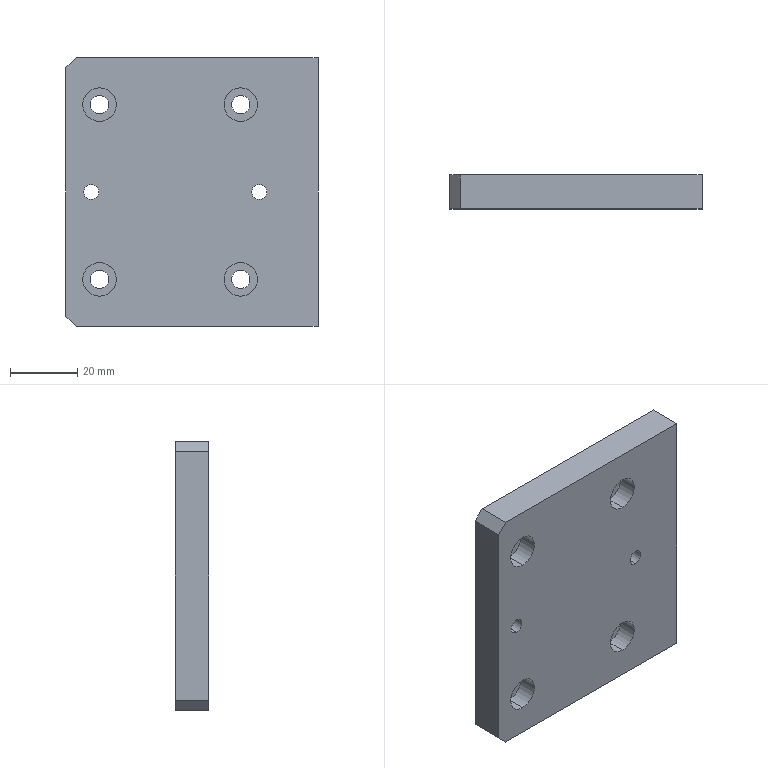Part | SolidWorks | features HoleWzd 3, Chamfer 1, Extrusion 1 | 1 solid | 46 faces | box 75 x 10 x 80 mm | volume 56721 mm3 | cylinder 28 | plane 14 | cone 4 | commonest cylinder face diameters 5.5 x8 10 x8 4.2 x4 4.5 x4 8 x4
STEP:
#1=CARTESIAN_POINT('',(-30.,0.4,-4.));
#2=VERTEX_POINT('',#1);
#3=CARTESIAN_POINT('',(-30.,0.4,4.));
#4=VERTEX_POINT('',#3);
#5=CARTESIAN_POINT('',(-30.,0.4,0.));
#6=DIRECTION('',(0.,1.,0.));
#7=DIRECTION('',(0.,0.,1.));
#8=AXIS2_PLACEMENT_3D('',#5,#6,#7);
#9=CIRCLE('',#8,4.);
#10=EDGE_CURVE('',#2,#4,#9,.T.);
#11=ORIENTED_EDGE('',*,*,#10,.F.);
#12=CARTESIAN_POINT('',(-30.,5.,-4.));
#13=VERTEX_POINT('',#12);
#14=CARTESIAN_POINT('',(-30.,5.,-4.));
#15=DIRECTION('',(0.,1.,0.));
#16=VECTOR('',#15,1000.);
#17=LINE('',#14,#16);
#18=EDGE_CURVE('',#2,#13,#17,.T.);
#19=ORIENTED_EDGE('',*,*,#18,.T.);
#20=CARTESIAN_POINT('',(-30.,5.,4.));
#21=VERTEX_POINT('',#20);
#22=CARTESIAN_POINT('',(-30.,5.,0.));
#23=DIRECTION('',(0.,1.,0.));
#24=DIRECTION('',(0.,0.,1.));
#25=AXIS2_PLACEMENT_3D('',#22,#23,#24);
#26=CIRCLE('',#25,4.);
#27=EDGE_CURVE('',#13,#21,#26,.T.);
#28=ORIENTED_EDGE('',*,*,#27,.T.);
#29=CARTESIAN_POINT('',(-30.,5.,4.));
#30=DIRECTION('',(0.,1.,0.));
#31=VECTOR('',#30,1000.);
#32=LINE('',#29,#31);
#33=EDGE_CURVE('',#4,#21,#32,.T.);
#34=ORIENTED_EDGE('',*,*,#33,.F.);
#35=EDGE_LOOP('',(#11,#19,#28,#34));
#36=FACE_OUTER_BOUND('',#35,.T.);
#37=CARTESIAN_POINT('',(-30.,5.,0.));
#38=DIRECTION('',(0.,1.,0.));
#39=DIRECTION('',(0.,0.,1.));
#40=AXIS2_PLACEMENT_3D('',#37,#38,#39);
#41=CYLINDRICAL_SURFACE('',#40,4.);
#42=ADVANCED_FACE('',(#36),#41,.F.);
#43=CARTESIAN_POINT('',(-30.,-5.,-2.25));
#44=VERTEX_POINT('',#43);
#45=CARTESIAN_POINT('',(-30.,-5.,2.25));
#46=VERTEX_POINT('',#45);
#47=CARTESIAN_POINT('',(-30.,-5.,0.));
#48=DIRECTION('',(0.,1.,0.));
#49=DIRECTION('',(0.,0.,1.));
#50=AXIS2_PLACEMENT_3D('',#47,#48,#49);
#51=CIRCLE('',#50,2.25);
#52=EDGE_CURVE('',#44,#46,#51,.T.);
#53=ORIENTED_EDGE('',*,*,#52,.F.);
#54=CARTESIAN_POINT('',(-30.,0.4,-2.25));
#55=VERTEX_POINT('',#54);
#56=CARTESIAN_POINT('',(-30.,5.,-2.25));
#57=DIRECTION('',(0.,1.,0.));
#58=VECTOR('',#57,1000.);
#59=LINE('',#56,#58);
#60=EDGE_CURVE('',#44,#55,#59,.T.);
#61=ORIENTED_EDGE('',*,*,#60,.T.);
#62=CARTESIAN_POINT('',(-30.,0.4,2.25));
#63=VERTEX_POINT('',#62);
#64=CARTESIAN_POINT('',(-30.,0.4,0.));
#65=DIRECTION('',(0.,1.,0.));
#66=DIRECTION('',(0.,0.,1.));
#67=AXIS2_PLACEMENT_3D('',#64,#65,#66);
#68=CIRCLE('',#67,2.25);
#69=EDGE_CURVE('',#55,#63,#68,.T.);
#70=ORIENTED_EDGE('',*,*,#69,.T.);
#71=CARTESIAN_POINT('',(-30.,5.,2.25));
#72=DIRECTION('',(0.,1.,0.));
#73=VECTOR('',#72,1000.);
#74=LINE('',#71,#73);
#75=EDGE_CURVE('',#46,#63,#74,.T.);
#76=ORIENTED_EDGE('',*,*,#75,.F.);
#77=EDGE_LOOP('',(#53,#61,#70,#76));
#78=FACE_OUTER_BOUND('',#77,.T.);
#79=CARTESIAN_POINT('',(-30.,5.,0.));
#80=DIRECTION('',(0.,1.,0.));
#81=DIRECTION('',(0.,0.,1.));
#82=AXIS2_PLACEMENT_3D('',#79,#80,#81);
#83=CYLINDRICAL_SURFACE('',#82,2.25);
#84=ADVANCED_FACE('',(#78),#83,.F.);
#85=CARTESIAN_POINT('',(20.,0.4,-4.));
#86=VERTEX_POINT('',#85);
#87=CARTESIAN_POINT('',(20.,0.4,4.));
#88=VERTEX_POINT('',#87);
#89=CARTESIAN_POINT('',(20.,0.4,0.));
#90=DIRECTION('',(0.,1.,0.));
#91=DIRECTION('',(0.,0.,1.));
#92=AXIS2_PLACEMENT_3D('',#89,#90,#91);
#93=CIRCLE('',#92,4.);
#94=EDGE_CURVE('',#86,#88,#93,.T.);
#95=ORIENTED_EDGE('',*,*,#94,.F.);
#96=CARTESIAN_POINT('',(20.,5.,-4.));
#97=VERTEX_POINT('',#96);
#98=CARTESIAN_POINT('',(20.,5.,-4.));
#99=DIRECTION('',(0.,1.,0.));
#100=VECTOR('',#99,1000.);
#101=LINE('',#98,#100);
#102=EDGE_CURVE('',#86,#97,#101,.T.);
#103=ORIENTED_EDGE('',*,*,#102,.T.);
#104=CARTESIAN_POINT('',(20.,5.,4.));
#105=VERTEX_POINT('',#104);
#106=CARTESIAN_POINT('',(20.,5.,0.));
#107=DIRECTION('',(0.,1.,0.));
#108=DIRECTION('',(0.,0.,1.));
#109=AXIS2_PLACEMENT_3D('',#106,#107,#108);
#110=CIRCLE('',#109,4.);
#111=EDGE_CURVE('',#97,#105,#110,.T.);
#112=ORIENTED_EDGE('',*,*,#111,.T.);
#113=CARTESIAN_POINT('',(20.,5.,4.));
#114=DIRECTION('',(0.,1.,0.));
#115=VECTOR('',#114,1000.);
#116=LINE('',#113,#115);
#117=EDGE_CURVE('',#88,#105,#116,.T.);
#118=ORIENTED_EDGE('',*,*,#117,.F.);
#119=EDGE_LOOP('',(#95,#103,#112,#118));
#120=FACE_OUTER_BOUND('',#119,.T.);
#121=CARTESIAN_POINT('',(20.,5.,0.));
#122=DIRECTION('',(0.,1.,0.));
#123=DIRECTION('',(0.,0.,1.));
#124=AXIS2_PLACEMENT_3D('',#121,#122,#123);
#125=CYLINDRICAL_SURFACE('',#124,4.);
#126=ADVANCED_FACE('',(#120),#125,.F.);
#127=CARTESIAN_POINT('',(20.,-5.,-2.25));
#128=VERTEX_POINT('',#127);
#129=CARTESIAN_POINT('',(20.,-5.,2.25));
#130=VERTEX_POINT('',#129);
#131=CARTESIAN_POINT('',(20.,-5.,0.));
#132=DIRECTION('',(0.,1.,0.));
#133=DIRECTION('',(0.,0.,1.));
#134=AXIS2_PLACEMENT_3D('',#131,#132,#133);
#135=CIRCLE('',#134,2.25);
#136=EDGE_CURVE('',#128,#130,#135,.T.);
#137=ORIENTED_EDGE('',*,*,#136,.F.);
#138=CARTESIAN_POINT('',(20.,0.4,-2.25));
#139=VERTEX_POINT('',#138);
#140=CARTESIAN_POINT('',(20.,5.,-2.25));
#141=DIRECTION('',(0.,1.,0.));
#142=VECTOR('',#141,1000.);
#143=LINE('',#140,#142);
#144=EDGE_CURVE('',#128,#139,#143,.T.);
#145=ORIENTED_EDGE('',*,*,#144,.T.);
#146=CARTESIAN_POINT('',(20.,0.4,2.25));
#147=VERTEX_POINT('',#146);
#148=CARTESIAN_POINT('',(20.,0.4,0.));
#149=DIRECTION('',(0.,1.,0.));
#150=DIRECTION('',(0.,0.,1.));
#151=AXIS2_PLACEMENT_3D('',#148,#149,#150);
#152=CIRCLE('',#151,2.25);
#153=EDGE_CURVE('',#139,#147,#152,.T.);
#154=ORIENTED_EDGE('',*,*,#153,.T.);
#155=CARTESIAN_POINT('',(20.,5.,2.25));
#156=DIRECTION('',(0.,1.,0.));
#157=VECTOR('',#156,1000.);
#158=LINE('',#155,#157);
#159=EDGE_CURVE('',#130,#147,#158,.T.);
#160=ORIENTED_EDGE('',*,*,#159,.F.);
#161=EDGE_LOOP('',(#137,#145,#154,#160));
#162=FACE_OUTER_BOUND('',#161,.T.);
#163=CARTESIAN_POINT('',(20.,5.,0.));
#164=DIRECTION('',(0.,1.,0.));
#165=DIRECTION('',(0.,0.,1.));
#166=AXIS2_PLACEMENT_3D('',#163,#164,#165);
#167=CYLINDRICAL_SURFACE('',#166,2.25);
#168=ADVANCED_FACE('',(#162),#167,.F.);
#169=CARTESIAN_POINT('',(-27.5,0.7,-21.));
#170=VERTEX_POINT('',#169);
#171=CARTESIAN_POINT('',(-27.5,0.7,-31.));
#172=VERTEX_POINT('',#171);
#173=CARTESIAN_POINT('',(-27.5,0.7,-26.));
#174=DIRECTION('',(0.,-1.,0.));
#175=DIRECTION('',(0.,0.,-1.));
#176=AXIS2_PLACEMENT_3D('',#173,#174,#175);
#177=CIRCLE('',#176,5.);
#178=EDGE_CURVE('',#170,#172,#177,.T.);
#179=ORIENTED_EDGE('',*,*,#178,.F.);
#180=CARTESIAN_POINT('',(-27.5,-5.,-21.));
#181=VERTEX_POINT('',#180);
#182=CARTESIAN_POINT('',(-27.5,-5.,-21.));
#183=DIRECTION('',(0.,-1.,0.));
#184=VECTOR('',#183,1000.);
#185=LINE('',#182,#184);
#186=EDGE_CURVE('',#170,#181,#185,.T.);
#187=ORIENTED_EDGE('',*,*,#186,.T.);
#188=CARTESIAN_POINT('',(-27.5,-5.,-31.));
#189=VERTEX_POINT('',#188);
#190=CARTESIAN_POINT('',(-27.5,-5.,-26.));
#191=DIRECTION('',(0.,-1.,0.));
#192=DIRECTION('',(0.,0.,-1.));
#193=AXIS2_PLACEMENT_3D('',#190,#191,#192);
#194=CIRCLE('',#193,5.);
#195=EDGE_CURVE('',#181,#189,#194,.T.);
#196=ORIENTED_EDGE('',*,*,#195,.T.);
#197=CARTESIAN_POINT('',(-27.5,-5.,-31.));
#198=DIRECTION('',(0.,-1.,0.));
#199=VECTOR('',#198,1000.);
#200=LINE('',#197,#199);
#201=EDGE_CURVE('',#172,#189,#200,.T.);
#202=ORIENTED_EDGE('',*,*,#201,.F.);
#203=EDGE_LOOP('',(#179,#187,#196,#202));
#204=FACE_OUTER_BOUND('',#203,.T.);
#205=CARTESIAN_POINT('',(-27.5,-5.,-26.));
#206=DIRECTION('',(0.,-1.,0.));
#207=DIRECTION('',(0.,0.,-1.));
#208=AXIS2_PLACEMENT_3D('',#205,#206,#207);
#209=CYLINDRICAL_SURFACE('',#208,5.);
#210=ADVANCED_FACE('',(#204),#209,.F.);
#211=CARTESIAN_POINT('',(-27.5,5.,-23.25));
#212=VERTEX_POINT('',#211);
#213=CARTESIAN_POINT('',(-27.5,5.,-28.75));
#214=VERTEX_POINT('',#213);
#215=CARTESIAN_POINT('',(-27.5,5.,-26.));
#216=DIRECTION('',(0.,-1.,0.));
#217=DIRECTION('',(0.,0.,-1.));
#218=AXIS2_PLACEMENT_3D('',#215,#216,#217);
#219=CIRCLE('',#218,2.75);
#220=EDGE_CURVE('',#212,#214,#219,.T.);
#221=ORIENTED_EDGE('',*,*,#220,.F.);
#222=CARTESIAN_POINT('',(-27.5,0.7,-23.25));
#223=VERTEX_POINT('',#222);
#224=CARTESIAN_POINT('',(-27.5,-5.,-23.25));
#225=DIRECTION('',(0.,-1.,0.));
#226=VECTOR('',#225,1000.);
#227=LINE('',#224,#226);
#228=EDGE_CURVE('',#212,#223,#227,.T.);
#229=ORIENTED_EDGE('',*,*,#228,.T.);
#230=CARTESIAN_POINT('',(-27.5,0.7,-28.75));
#231=VERTEX_POINT('',#230);
#232=CARTESIAN_POINT('',(-27.5,0.7,-26.));
#233=DIRECTION('',(0.,-1.,0.));
#234=DIRECTION('',(0.,0.,-1.));
#235=AXIS2_PLACEMENT_3D('',#232,#233,#234);
#236=CIRCLE('',#235,2.75);
#237=EDGE_CURVE('',#223,#231,#236,.T.);
#238=ORIENTED_EDGE('',*,*,#237,.T.);
#239=CARTESIAN_POINT('',(-27.5,-5.,-28.75));
#240=DIRECTION('',(0.,-1.,0.));
#241=VECTOR('',#240,1000.);
#242=LINE('',#239,#241);
#243=EDGE_CURVE('',#214,#231,#242,.T.);
#244=ORIENTED_EDGE('',*,*,#243,.F.);
#245=EDGE_LOOP('',(#221,#229,#238,#244));
#246=FACE_OUTER_BOUND('',#245,.T.);
#247=CARTESIAN_POINT('',(-27.5,-5.,-26.));
#248=DIRECTION('',(0.,-1.,0.));
#249=DIRECTION('',(0.,0.,-1.));
#250=AXIS2_PLACEMENT_3D('',#247,#248,#249);
#251=CYLINDRICAL_SURFACE('',#250,2.75);
#252=ADVANCED_FACE('',(#246),#251,.F.);
#253=CARTESIAN_POINT('',(14.5,0.7,-21.));
#254=VERTEX_POINT('',#253);
#255=CARTESIAN_POINT('',(14.5,0.7,-31.));
#256=VERTEX_POINT('',#255);
#257=CARTESIAN_POINT('',(14.5,0.7,-26.));
#258=DIRECTION('',(0.,-1.,0.));
#259=DIRECTION('',(0.,0.,-1.));
#260=AXIS2_PLACEMENT_3D('',#257,#258,#259);
#261=CIRCLE('',#260,5.);
#262=EDGE_CURVE('',#254,#256,#261,.T.);
#263=ORIENTED_EDGE('',*,*,#262,.F.);
#264=CARTESIAN_POINT('',(14.5,-5.,-21.));
#265=VERTEX_POINT('',#264);
#266=CARTESIAN_POINT('',(14.5,-5.,-21.));
#267=DIRECTION('',(0.,-1.,0.));
#268=VECTOR('',#267,1000.);
#269=LINE('',#266,#268);
#270=EDGE_CURVE('',#254,#265,#269,.T.);
#271=ORIENTED_EDGE('',*,*,#270,.T.);
#272=CARTESIAN_POINT('',(14.5,-5.,-31.));
#273=VERTEX_POINT('',#272);
#274=CARTESIAN_POINT('',(14.5,-5.,-26.));
#275=DIRECTION('',(0.,-1.,0.));
#276=DIRECTION('',(0.,0.,-1.));
#277=AXIS2_PLACEMENT_3D('',#274,#275,#276);
#278=CIRCLE('',#277,5.);
#279=EDGE_CURVE('',#265,#273,#278,.T.);
#280=ORIENTED_EDGE('',*,*,#279,.T.);
#281=CARTESIAN_POINT('',(14.5,-5.,-31.));
#282=DIRECTION('',(0.,-1.,0.));
#283=VECTOR('',#282,1000.);
#284=LINE('',#281,#283);
#285=EDGE_CURVE('',#256,#273,#284,.T.);
#286=ORIENTED_EDGE('',*,*,#285,.F.);
#287=EDGE_LOOP('',(#263,#271,#280,#286));
#288=FACE_OUTER_BOUND('',#287,.T.);
#289=CARTESIAN_POINT('',(14.5,-5.,-26.));
#290=DIRECTION('',(0.,-1.,0.));
#291=DIRECTION('',(0.,0.,-1.));
#292=AXIS2_PLACEMENT_3D('',#289,#290,#291);
#293=CYLINDRICAL_SURFACE('',#292,5.);
#294=ADVANCED_FACE('',(#288),#293,.F.);
#295=CARTESIAN_POINT('',(14.5,5.,-23.25));
#296=VERTEX_POINT('',#295);
#297=CARTESIAN_POINT('',(14.5,5.,-28.75));
#298=VERTEX_POINT('',#297);
#299=CARTESIAN_POINT('',(14.5,5.,-26.));
#300=DIRECTION('',(0.,-1.,0.));
#301=DIRECTION('',(0.,0.,-1.));
#302=AXIS2_PLACEMENT_3D('',#299,#300,#301);
#303=CIRCLE('',#302,2.75);
#304=EDGE_CURVE('',#296,#298,#303,.T.);
#305=ORIENTED_EDGE('',*,*,#304,.F.);
#306=CARTESIAN_POINT('',(14.5,0.7,-23.25));
#307=VERTEX_POINT('',#306);
#308=CARTESIAN_POINT('',(14.5,-5.,-23.25));
#309=DIRECTION('',(0.,-1.,0.));
#310=VECTOR('',#309,1000.);
#311=LINE('',#308,#310);
#312=EDGE_CURVE('',#296,#307,#311,.T.);
#313=ORIENTED_EDGE('',*,*,#312,.T.);
#314=CARTESIAN_POINT('',(14.5,0.7,-28.75));
#315=VERTEX_POINT('',#314);
#316=CARTESIAN_POINT('',(14.5,0.7,-26.));
#317=DIRECTION('',(0.,-1.,0.));
#318=DIRECTION('',(0.,0.,-1.));
#319=AXIS2_PLACEMENT_3D('',#316,#317,#318);
#320=CIRCLE('',#319,2.75);
#321=EDGE_CURVE('',#307,#315,#320,.T.);
#322=ORIENTED_EDGE('',*,*,#321,.T.);
#323=CARTESIAN_POINT('',(14.5,-5.,-28.75));
#324=DIRECTION('',(0.,-1.,0.));
#325=VECTOR('',#324,1000.);
#326=LINE('',#323,#325);
#327=EDGE_CURVE('',#298,#315,#326,.T.);
#328=ORIENTED_EDGE('',*,*,#327,.F.);
#329=EDGE_LOOP('',(#305,#313,#322,#328));
#330=FACE_OUTER_BOUND('',#329,.T.);
#331=CARTESIAN_POINT('',(14.5,-5.,-26.));
#332=DIRECTION('',(0.,-1.,0.));
#333=DIRECTION('',(0.,0.,-1.));
#334=AXIS2_PLACEMENT_3D('',#331,#332,#333);
#335=CYLINDRICAL_SURFACE('',#334,2.75);
#336=ADVANCED_FACE('',(#330),#335,.F.);
#337=CARTESIAN_POINT('',(14.5,0.7,31.));
#338=VERTEX_POINT('',#337);
#339=CARTESIAN_POINT('',(14.5,0.7,21.));
#340=VERTEX_POINT('',#339);
#341=CARTESIAN_POINT('',(14.5,0.7,26.));
#342=DIRECTION('',(0.,-1.,0.));
#343=DIRECTION('',(0.,0.,-1.));
#344=AXIS2_PLACEMENT_3D('',#341,#342,#343);
#345=CIRCLE('',#344,5.);
#346=EDGE_CURVE('',#338,#340,#345,.T.);
#347=ORIENTED_EDGE('',*,*,#346,.F.);
#348=CARTESIAN_POINT('',(14.5,-5.,31.));
#349=VERTEX_POINT('',#348);
#350=CARTESIAN_POINT('',(14.5,-5.,31.));
#351=DIRECTION('',(0.,-1.,0.));
#352=VECTOR('',#351,1000.);
#353=LINE('',#350,#352);
#354=EDGE_CURVE('',#338,#349,#353,.T.);
#355=ORIENTED_EDGE('',*,*,#354,.T.);
#356=CARTESIAN_POINT('',(14.5,-5.,21.));
#357=VERTEX_POINT('',#356);
#358=CARTESIAN_POINT('',(14.5,-5.,26.));
#359=DIRECTION('',(0.,-1.,0.));
#360=DIRECTION('',(0.,0.,-1.));
#361=AXIS2_PLACEMENT_3D('',#358,#359,#360);
#362=CIRCLE('',#361,5.);
#363=EDGE_CURVE('',#349,#357,#362,.T.);
#364=ORIENTED_EDGE('',*,*,#363,.T.);
#365=CARTESIAN_POINT('',(14.5,-5.,21.));
#366=DIRECTION('',(0.,-1.,0.));
#367=VECTOR('',#366,1000.);
#368=LINE('',#365,#367);
#369=EDGE_CURVE('',#340,#357,#368,.T.);
#370=ORIENTED_EDGE('',*,*,#369,.F.);
#371=EDGE_LOOP('',(#347,#355,#364,#370));
#372=FACE_OUTER_BOUND('',#371,.T.);
#373=CARTESIAN_POINT('',(14.5,-5.,26.));
#374=DIRECTION('',(0.,-1.,0.));
#375=DIRECTION('',(0.,0.,-1.));
#376=AXIS2_PLACEMENT_3D('',#373,#374,#375);
#377=CYLINDRICAL_SURFACE('',#376,5.);
#378=ADVANCED_FACE('',(#372),#377,.F.);
#379=CARTESIAN_POINT('',(14.5,5.,28.75));
#380=VERTEX_POINT('',#379);
#381=CARTESIAN_POINT('',(14.5,5.,23.25));
#382=VERTEX_POINT('',#381);
#383=CARTESIAN_POINT('',(14.5,5.,26.));
#384=DIRECTION('',(0.,-1.,0.));
#385=DIRECTION('',(0.,0.,-1.));
#386=AXIS2_PLACEMENT_3D('',#383,#384,#385);
#387=CIRCLE('',#386,2.75);
#388=EDGE_CURVE('',#380,#382,#387,.T.);
#389=ORIENTED_EDGE('',*,*,#388,.F.);
#390=CARTESIAN_POINT('',(14.5,0.7,28.75));
#391=VERTEX_POINT('',#390);
#392=CARTESIAN_POINT('',(14.5,-5.,28.75));
#393=DIRECTION('',(0.,-1.,0.));
#394=VECTOR('',#393,1000.);
#395=LINE('',#392,#394);
#396=EDGE_CURVE('',#380,#391,#395,.T.);
#397=ORIENTED_EDGE('',*,*,#396,.T.);
#398=CARTESIAN_POINT('',(14.5,0.7,23.25));
#399=VERTEX_POINT('',#398);
#400=CARTESIAN_POINT('',(14.5,0.7,26.));
#401=DIRECTION('',(0.,-1.,0.));
#402=DIRECTION('',(0.,0.,-1.));
#403=AXIS2_PLACEMENT_3D('',#400,#401,#402);
#404=CIRCLE('',#403,2.75);
#405=EDGE_CURVE('',#391,#399,#404,.T.);
#406=ORIENTED_EDGE('',*,*,#405,.T.);
#407=CARTESIAN_POINT('',(14.5,-5.,23.25));
#408=DIRECTION('',(0.,-1.,0.));
#409=VECTOR('',#408,1000.);
#410=LINE('',#407,#409);
#411=EDGE_CURVE('',#382,#399,#410,.T.);
#412=ORIENTED_EDGE('',*,*,#411,.F.);
#413=EDGE_LOOP('',(#389,#397,#406,#412));
#414=FACE_OUTER_BOUND('',#413,.T.);
#415=CARTESIAN_POINT('',(14.5,-5.,26.));
#416=DIRECTION('',(0.,-1.,0.));
#417=DIRECTION('',(0.,0.,-1.));
#418=AXIS2_PLACEMENT_3D('',#415,#416,#417);
#419=CYLINDRICAL_SURFACE('',#418,2.75);
#420=ADVANCED_FACE('',(#414),#419,.F.);
#421=CARTESIAN_POINT('',(-27.5,0.7,31.));
#422=VERTEX_POINT('',#421);
#423=CARTESIAN_POINT('',(-27.5,0.7,21.));
#424=VERTEX_POINT('',#423);
#425=CARTESIAN_POINT('',(-27.5,0.7,26.));
#426=DIRECTION('',(0.,-1.,0.));
#427=DIRECTION('',(0.,0.,-1.));
#428=AXIS2_PLACEMENT_3D('',#425,#426,#427);
#429=CIRCLE('',#428,5.);
#430=EDGE_CURVE('',#422,#424,#429,.T.);
#431=ORIENTED_EDGE('',*,*,#430,.F.);
#432=CARTESIAN_POINT('',(-27.5,-5.,31.));
#433=VERTEX_POINT('',#432);
#434=CARTESIAN_POINT('',(-27.5,-5.,31.));
#435=DIRECTION('',(0.,-1.,0.));
#436=VECTOR('',#435,1000.);
#437=LINE('',#434,#436);
#438=EDGE_CURVE('',#422,#433,#437,.T.);
#439=ORIENTED_EDGE('',*,*,#438,.T.);
#440=CARTESIAN_POINT('',(-27.5,-5.,21.));
#441=VERTEX_POINT('',#440);
#442=CARTESIAN_POINT('',(-27.5,-5.,26.));
#443=DIRECTION('',(0.,-1.,0.));
#444=DIRECTION('',(0.,0.,-1.));
#445=AXIS2_PLACEMENT_3D('',#442,#443,#444);
#446=CIRCLE('',#445,5.);
#447=EDGE_CURVE('',#433,#441,#446,.T.);
#448=ORIENTED_EDGE('',*,*,#447,.T.);
#449=CARTESIAN_POINT('',(-27.5,-5.,21.));
#450=DIRECTION('',(0.,-1.,0.));
#451=VECTOR('',#450,1000.);
#452=LINE('',#449,#451);
#453=EDGE_CURVE('',#424,#441,#452,.T.);
#454=ORIENTED_EDGE('',*,*,#453,.F.);
#455=EDGE_LOOP('',(#431,#439,#448,#454));
#456=FACE_OUTER_BOUND('',#455,.T.);
#457=CARTESIAN_POINT('',(-27.5,-5.,26.));
#458=DIRECTION('',(0.,-1.,0.));
#459=DIRECTION('',(0.,0.,-1.));
#460=AXIS2_PLACEMENT_3D('',#457,#458,#459);
#461=CYLINDRICAL_SURFACE('',#460,5.);
#462=ADVANCED_FACE('',(#456),#461,.F.);
#463=CARTESIAN_POINT('',(-27.5,5.,28.75));
#464=VERTEX_POINT('',#463);
#465=CARTESIAN_POINT('',(-27.5,5.,23.25));
#466=VERTEX_POINT('',#465);
#467=CARTESIAN_POINT('',(-27.5,5.,26.));
#468=DIRECTION('',(0.,-1.,0.));
#469=DIRECTION('',(0.,0.,-1.));
#470=AXIS2_PLACEMENT_3D('',#467,#468,#469);
#471=CIRCLE('',#470,2.75);
#472=EDGE_CURVE('',#464,#466,#471,.T.);
#473=ORIENTED_EDGE('',*,*,#472,.F.);
#474=CARTESIAN_POINT('',(-27.5,0.7,28.75));
#475=VERTEX_POINT('',#474);
#476=CARTESIAN_POINT('',(-27.5,-5.,28.75));
#477=DIRECTION('',(0.,-1.,0.));
#478=VECTOR('',#477,1000.);
#479=LINE('',#476,#478);
#480=EDGE_CURVE('',#464,#475,#479,.T.);
#481=ORIENTED_EDGE('',*,*,#480,.T.);
#482=CARTESIAN_POINT('',(-27.5,0.7,23.25));
#483=VERTEX_POINT('',#482);
#484=CARTESIAN_POINT('',(-27.5,0.7,26.));
#485=DIRECTION('',(0.,-1.,0.));
#486=DIRECTION('',(0.,0.,-1.));
#487=AXIS2_PLACEMENT_3D('',#484,#485,#486);
#488=CIRCLE('',#487,2.75);
#489=EDGE_CURVE('',#475,#483,#488,.T.);
#490=ORIENTED_EDGE('',*,*,#489,.T.);
#491=CARTESIAN_POINT('',(-27.5,-5.,23.25));
#492=DIRECTION('',(0.,-1.,0.));
#493=VECTOR('',#492,1000.);
#494=LINE('',#491,#493);
#495=EDGE_CURVE('',#466,#483,#494,.T.);
#496=ORIENTED_EDGE('',*,*,#495,.F.);
#497=EDGE_LOOP('',(#473,#481,#490,#496));
#498=FACE_OUTER_BOUND('',#497,.T.);
#499=CARTESIAN_POINT('',(-27.5,-5.,26.));
#500=DIRECTION('',(0.,-1.,0.));
#501=DIRECTION('',(0.,0.,-1.));
#502=AXIS2_PLACEMENT_3D('',#499,#500,#501);
#503=CYLINDRICAL_SURFACE('',#502,2.75);
#504=ADVANCED_FACE('',(#498),#503,.F.);
#505=CARTESIAN_POINT('',(25.1,0.,32.1));
#506=VERTEX_POINT('',#505);
#507=CARTESIAN_POINT('',(25.1,0.,27.9));
#508=VERTEX_POINT('',#507);
#509=CARTESIAN_POINT('',(25.1,0.,30.));
#510=DIRECTION('',(1.,0.,0.));
#511=DIRECTION('',(0.,0.,-1.));
#512=AXIS2_PLACEMENT_3D('',#509,#510,#511);
#513=CIRCLE('',#512,2.1);
#514=EDGE_CURVE('',#506,#508,#513,.T.);
#515=ORIENTED_EDGE('',*,*,#514,.F.);
#516=CARTESIAN_POINT('',(37.5,0.,32.1));
#517=VERTEX_POINT('',#516);
#518=CARTESIAN_POINT('',(37.5,0.,32.1));
#519=DIRECTION('',(1.,0.,0.));
#520=VECTOR('',#519,1000.);
#521=LINE('',#518,#520);
#522=EDGE_CURVE('',#506,#517,#521,.T.);
#523=ORIENTED_EDGE('',*,*,#522,.T.);
#524=CARTESIAN_POINT('',(37.5,0.,27.9));
#525=VERTEX_POINT('',#524);
#526=CARTESIAN_POINT('',(37.5,0.,30.));
#527=DIRECTION('',(1.,0.,0.));
#528=DIRECTION('',(0.,0.,-1.));
#529=AXIS2_PLACEMENT_3D('',#526,#527,#528);
#530=CIRCLE('',#529,2.1);
#531=EDGE_CURVE('',#517,#525,#530,.T.);
#532=ORIENTED_EDGE('',*,*,#531,.T.);
#533=CARTESIAN_POINT('',(37.5,0.,27.9));
#534=DIRECTION('',(1.,0.,0.));
#535=VECTOR('',#534,1000.);
#536=LINE('',#533,#535);
#537=EDGE_CURVE('',#508,#525,#536,.T.);
#538=ORIENTED_EDGE('',*,*,#537,.F.);
#539=EDGE_LOOP('',(#515,#523,#532,#538));
#540=FACE_OUTER_BOUND('',#539,.T.);
#541=CARTESIAN_POINT('',(37.5,0.,30.));
#542=DIRECTION('',(1.,0.,0.));
#543=DIRECTION('',(0.,0.,-1.));
#544=AXIS2_PLACEMENT_3D('',#541,#542,#543);
#545=CYLINDRICAL_SURFACE('',#544,2.1);
#546=ADVANCED_FACE('',(#540),#545,.F.);
#547=CARTESIAN_POINT('',(23.838,0.,30.));
#548=VERTEX_POINT('',#547);
#549=CARTESIAN_POINT('',(25.1,0.,27.9));
#550=DIRECTION('',(0.515,0.,-0.8572));
#551=VECTOR('',#550,1000.);
#552=LINE('',#549,#551);
#553=EDGE_CURVE('',#548,#508,#552,.T.);
#554=ORIENTED_EDGE('',*,*,#553,.F.);
#555=CARTESIAN_POINT('',(25.1,0.,32.1));
#556=DIRECTION('',(0.515,0.,0.8572));
#557=VECTOR('',#556,1000.);
#558=LINE('',#555,#557);
#559=EDGE_CURVE('',#548,#506,#558,.T.);
#560=ORIENTED_EDGE('',*,*,#559,.T.);
#561=ORIENTED_EDGE('',*,*,#514,.T.);
#562=EDGE_LOOP('',(#554,#560,#561));
#563=FACE_OUTER_BOUND('',#562,.T.);
#564=CARTESIAN_POINT('',(25.1,0.,30.));
#565=DIRECTION('',(1.,0.,0.));
#566=DIRECTION('',(0.,0.,-1.));
#567=AXIS2_PLACEMENT_3D('',#564,#565,#566);
#568=CONICAL_SURFACE('',#567,2.1,1.03);
#569=ADVANCED_FACE('',(#563),#568,.F.);
#570=CARTESIAN_POINT('',(25.1,0.,-27.9));
#571=VERTEX_POINT('',#570);
#572=CARTESIAN_POINT('',(25.1,0.,-32.1));
#573=VERTEX_POINT('',#572);
#574=CARTESIAN_POINT('',(25.1,0.,-30.));
#575=DIRECTION('',(1.,0.,0.));
#576=DIRECTION('',(0.,0.,-1.));
#577=AXIS2_PLACEMENT_3D('',#574,#575,#576);
#578=CIRCLE('',#577,2.1);
#579=EDGE_CURVE('',#571,#573,#578,.T.);
#580=ORIENTED_EDGE('',*,*,#579,.F.);
#581=CARTESIAN_POINT('',(37.5,0.,-27.9));
#582=VERTEX_POINT('',#581);
#583=CARTESIAN_POINT('',(37.5,0.,-27.9));
#584=DIRECTION('',(1.,0.,0.));
#585=VECTOR('',#584,1000.);
#586=LINE('',#583,#585);
#587=EDGE_CURVE('',#571,#582,#586,.T.);
#588=ORIENTED_EDGE('',*,*,#587,.T.);
#589=CARTESIAN_POINT('',(37.5,0.,-32.1));
#590=VERTEX_POINT('',#589);
#591=CARTESIAN_POINT('',(37.5,0.,-30.));
#592=DIRECTION('',(1.,0.,0.));
#593=DIRECTION('',(0.,0.,-1.));
#594=AXIS2_PLACEMENT_3D('',#591,#592,#593);
#595=CIRCLE('',#594,2.1);
#596=EDGE_CURVE('',#582,#590,#595,.T.);
#597=ORIENTED_EDGE('',*,*,#596,.T.);
#598=CARTESIAN_POINT('',(37.5,0.,-32.1));
#599=DIRECTION('',(1.,0.,0.));
#600=VECTOR('',#599,1000.);
#601=LINE('',#598,#600);
#602=EDGE_CURVE('',#573,#590,#601,.T.);
#603=ORIENTED_EDGE('',*,*,#602,.F.);
#604=EDGE_LOOP('',(#580,#588,#597,#603));
#605=FACE_OUTER_BOUND('',#604,.T.);
#606=CARTESIAN_POINT('',(37.5,0.,-30.));
#607=DIRECTION('',(1.,0.,0.));
#608=DIRECTION('',(0.,0.,-1.));
#609=AXIS2_PLACEMENT_3D('',#606,#607,#608);
#610=CYLINDRICAL_SURFACE('',#609,2.1);
#611=ADVANCED_FACE('',(#605),#610,.F.);
#612=CARTESIAN_POINT('',(23.838,0.,-30.));
#613=VERTEX_POINT('',#612);
#614=CARTESIAN_POINT('',(25.1,0.,-32.1));
#615=DIRECTION('',(0.515,0.,-0.8572));
#616=VECTOR('',#615,1000.);
#617=LINE('',#614,#616);
#618=EDGE_CURVE('',#613,#573,#617,.T.);
#619=ORIENTED_EDGE('',*,*,#618,.F.);
#620=CARTESIAN_POINT('',(25.1,0.,-27.9));
#621=DIRECTION('',(0.515,0.,0.8572));
#622=VECTOR('',#621,1000.);
#623=LINE('',#620,#622);
#624=EDGE_CURVE('',#613,#571,#623,.T.);
#625=ORIENTED_EDGE('',*,*,#624,.T.);
#626=ORIENTED_EDGE('',*,*,#579,.T.);
#627=EDGE_LOOP('',(#619,#625,#626));
#628=FACE_OUTER_BOUND('',#627,.T.);
#629=CARTESIAN_POINT('',(25.1,0.,-30.));
#630=DIRECTION('',(1.,0.,0.));
#631=DIRECTION('',(0.,0.,-1.));
#632=AXIS2_PLACEMENT_3D('',#629,#630,#631);
#633=CONICAL_SURFACE('',#632,2.1,1.03);
#634=ADVANCED_FACE('',(#628),#633,.F.);
#635=CARTESIAN_POINT('',(-30.,5.,0.));
#636=DIRECTION('',(0.,1.,0.));
#637=DIRECTION('',(0.,0.,1.));
#638=AXIS2_PLACEMENT_3D('',#635,#636,#637);
#639=CIRCLE('',#638,4.);
#640=EDGE_CURVE('',#21,#13,#639,.T.);
#641=ORIENTED_EDGE('',*,*,#640,.F.);
#642=ORIENTED_EDGE('',*,*,#27,.F.);
#643=EDGE_LOOP('',(#641,#642));
#644=FACE_BOUND('',#643,.T.);
#645=CARTESIAN_POINT('',(-27.5,5.,-26.));
#646=DIRECTION('',(0.,-1.,0.));
#647=DIRECTION('',(0.,0.,-1.));
#648=AXIS2_PLACEMENT_3D('',#645,#646,#647);
#649=CIRCLE('',#648,2.75);
#650=EDGE_CURVE('',#214,#212,#649,.T.);
#651=ORIENTED_EDGE('',*,*,#650,.T.);
#652=ORIENTED_EDGE('',*,*,#220,.T.);
#653=EDGE_LOOP('',(#651,#652));
#654=FACE_BOUND('',#653,.T.);
#655=CARTESIAN_POINT('',(14.5,5.,-26.));
#656=DIRECTION('',(0.,-1.,0.));
#657=DIRECTION('',(0.,0.,-1.));
#658=AXIS2_PLACEMENT_3D('',#655,#656,#657);
#659=CIRCLE('',#658,2.75);
#660=EDGE_CURVE('',#298,#296,#659,.T.);
#661=ORIENTED_EDGE('',*,*,#660,.T.);
#662=ORIENTED_EDGE('',*,*,#304,.T.);
#663=EDGE_LOOP('',(#661,#662));
#664=FACE_BOUND('',#663,.T.);
#665=CARTESIAN_POINT('',(14.5,5.,26.));
#666=DIRECTION('',(0.,-1.,0.));
#667=DIRECTION('',(0.,0.,-1.));
#668=AXIS2_PLACEMENT_3D('',#665,#666,#667);
#669=CIRCLE('',#668,2.75);
#670=EDGE_CURVE('',#382,#380,#669,.T.);
#671=ORIENTED_EDGE('',*,*,#670,.T.);
#672=ORIENTED_EDGE('',*,*,#388,.T.);
#673=EDGE_LOOP('',(#671,#672));
#674=FACE_BOUND('',#673,.T.);
#675=CARTESIAN_POINT('',(-27.5,5.,26.));
#676=DIRECTION('',(0.,-1.,0.));
#677=DIRECTION('',(0.,0.,-1.));
#678=AXIS2_PLACEMENT_3D('',#675,#676,#677);
#679=CIRCLE('',#678,2.75);
#680=EDGE_CURVE('',#466,#464,#679,.T.);
#681=ORIENTED_EDGE('',*,*,#680,.T.);
#682=ORIENTED_EDGE('',*,*,#472,.T.);
#683=EDGE_LOOP('',(#681,#682));
#684=FACE_BOUND('',#683,.T.);
#685=CARTESIAN_POINT('',(-37.5,5.,-37.));
#686=VERTEX_POINT('',#685);
#687=CARTESIAN_POINT('',(-37.5,5.,37.));
#688=VERTEX_POINT('',#687);
#689=CARTESIAN_POINT('',(-37.5,5.,40.));
#690=DIRECTION('',(0.,0.,1.));
#691=VECTOR('',#690,1000.);
#692=LINE('',#689,#691);
#693=EDGE_CURVE('',#686,#688,#692,.T.);
#694=ORIENTED_EDGE('',*,*,#693,.T.);
#695=CARTESIAN_POINT('',(-34.5,5.,40.));
#696=VERTEX_POINT('',#695);
#697=CARTESIAN_POINT('',(-34.5,5.,40.));
#698=DIRECTION('',(0.7071,0.,0.7071));
#699=VECTOR('',#698,1000.);
#700=LINE('',#697,#699);
#701=EDGE_CURVE('',#688,#696,#700,.T.);
#702=ORIENTED_EDGE('',*,*,#701,.T.);
#703=CARTESIAN_POINT('',(37.5,5.,40.));
#704=VERTEX_POINT('',#703);
#705=CARTESIAN_POINT('',(-37.5,5.,40.));
#706=DIRECTION('',(1.,0.,0.));
#707=VECTOR('',#706,1000.);
#708=LINE('',#705,#707);
#709=EDGE_CURVE('',#696,#704,#708,.T.);
#710=ORIENTED_EDGE('',*,*,#709,.T.);
#711=CARTESIAN_POINT('',(37.5,5.,-40.));
#712=VERTEX_POINT('',#711);
#713=CARTESIAN_POINT('',(37.5,5.,40.));
#714=DIRECTION('',(0.,0.,-1.));
#715=VECTOR('',#714,1000.);
#716=LINE('',#713,#715);
#717=EDGE_CURVE('',#704,#712,#716,.T.);
#718=ORIENTED_EDGE('',*,*,#717,.T.);
#719=CARTESIAN_POINT('',(-34.5,5.,-40.));
#720=VERTEX_POINT('',#719);
#721=CARTESIAN_POINT('',(-37.5,5.,-40.));
#722=DIRECTION('',(-1.,0.,0.));
#723=VECTOR('',#722,1000.);
#724=LINE('',#721,#723);
#725=EDGE_CURVE('',#712,#720,#724,.T.);
#726=ORIENTED_EDGE('',*,*,#725,.T.);
#727=CARTESIAN_POINT('',(-37.5,5.,-37.));
#728=DIRECTION('',(-0.7071,0.,0.7071));
#729=VECTOR('',#728,1000.);
#730=LINE('',#727,#729);
#731=EDGE_CURVE('',#720,#686,#730,.T.);
#732=ORIENTED_EDGE('',*,*,#731,.T.);
#733=EDGE_LOOP('',(#694,#702,#710,#718,#726,#732));
#734=FACE_OUTER_BOUND('',#733,.T.);
#735=CARTESIAN_POINT('',(20.,5.,0.));
#736=DIRECTION('',(0.,1.,0.));
#737=DIRECTION('',(0.,0.,1.));
#738=AXIS2_PLACEMENT_3D('',#735,#736,#737);
#739=CIRCLE('',#738,4.);
#740=EDGE_CURVE('',#105,#97,#739,.T.);
#741=ORIENTED_EDGE('',*,*,#740,.F.);
#742=ORIENTED_EDGE('',*,*,#111,.F.);
#743=EDGE_LOOP('',(#741,#742));
#744=FACE_BOUND('',#743,.T.);
#745=CARTESIAN_POINT('',(0.,5.,0.));
#746=DIRECTION('',(0.,-1.,0.));
#747=DIRECTION('',(0.,0.,-1.));
#748=AXIS2_PLACEMENT_3D('',#745,#746,#747);
#749=PLANE('',#748);
#750=ADVANCED_FACE('',(#644,#654,#664,#674,#684,#734,#744),#749,.F.);
#751=CARTESIAN_POINT('',(-30.,-5.,0.));
#752=DIRECTION('',(0.,1.,0.));
#753=DIRECTION('',(0.,0.,1.));
#754=AXIS2_PLACEMENT_3D('',#751,#752,#753);
#755=CIRCLE('',#754,2.25);
#756=EDGE_CURVE('',#46,#44,#755,.T.);
#757=ORIENTED_EDGE('',*,*,#756,.T.);
#758=ORIENTED_EDGE('',*,*,#52,.T.);
#759=EDGE_LOOP('',(#757,#758));
#760=FACE_BOUND('',#759,.T.);
#761=CARTESIAN_POINT('',(-34.5,-5.,40.));
#762=VERTEX_POINT('',#761);
#763=CARTESIAN_POINT('',(37.5,-5.,40.));
#764=VERTEX_POINT('',#763);
#765=CARTESIAN_POINT('',(-37.5,-5.,40.));
#766=DIRECTION('',(1.,0.,0.));
#767=VECTOR('',#766,1000.);
#768=LINE('',#765,#767);
#769=EDGE_CURVE('',#762,#764,#768,.T.);
#770=ORIENTED_EDGE('',*,*,#769,.F.);
#771=CARTESIAN_POINT('',(-37.5,-5.,37.));
#772=VERTEX_POINT('',#771);
#773=CARTESIAN_POINT('',(-37.25,-5.,37.25));
#774=DIRECTION('',(-0.7071,0.,-0.7071));
#775=VECTOR('',#774,1000.);
#776=LINE('',#773,#775);
#777=EDGE_CURVE('',#762,#772,#776,.T.);
#778=ORIENTED_EDGE('',*,*,#777,.T.);
#779=CARTESIAN_POINT('',(-37.5,-5.,-37.));
#780=VERTEX_POINT('',#779);
#781=CARTESIAN_POINT('',(-37.5,-5.,40.));
#782=DIRECTION('',(0.,0.,1.));
#783=VECTOR('',#782,1000.);
#784=LINE('',#781,#783);
#785=EDGE_CURVE('',#780,#772,#784,.T.);
#786=ORIENTED_EDGE('',*,*,#785,.F.);
#787=CARTESIAN_POINT('',(-34.5,-5.,-40.));
#788=VERTEX_POINT('',#787);
#789=CARTESIAN_POINT('',(-37.25,-5.,-37.25));
#790=DIRECTION('',(0.7071,0.,-0.7071));
#791=VECTOR('',#790,1000.);
#792=LINE('',#789,#791);
#793=EDGE_CURVE('',#780,#788,#792,.T.);
#794=ORIENTED_EDGE('',*,*,#793,.T.);
#795=CARTESIAN_POINT('',(37.5,-5.,-40.));
#796=VERTEX_POINT('',#795);
#797=CARTESIAN_POINT('',(-37.5,-5.,-40.));
#798=DIRECTION('',(-1.,0.,0.));
#799=VECTOR('',#798,1000.);
#800=LINE('',#797,#799);
#801=EDGE_CURVE('',#796,#788,#800,.T.);
#802=ORIENTED_EDGE('',*,*,#801,.F.);
#803=CARTESIAN_POINT('',(37.5,-5.,40.));
#804=DIRECTION('',(0.,0.,-1.));
#805=VECTOR('',#804,1000.);
#806=LINE('',#803,#805);
#807=EDGE_CURVE('',#764,#796,#806,.T.);
#808=ORIENTED_EDGE('',*,*,#807,.F.);
#809=EDGE_LOOP('',(#770,#778,#786,#794,#802,#808));
#810=FACE_OUTER_BOUND('',#809,.T.);
#811=CARTESIAN_POINT('',(-27.5,-5.,26.));
#812=DIRECTION('',(0.,-1.,0.));
#813=DIRECTION('',(0.,0.,-1.));
#814=AXIS2_PLACEMENT_3D('',#811,#812,#813);
#815=CIRCLE('',#814,5.);
#816=EDGE_CURVE('',#441,#433,#815,.T.);
#817=ORIENTED_EDGE('',*,*,#816,.F.);
#818=ORIENTED_EDGE('',*,*,#447,.F.);
#819=EDGE_LOOP('',(#817,#818));
#820=FACE_BOUND('',#819,.T.);
#821=CARTESIAN_POINT('',(14.5,-5.,26.));
#822=DIRECTION('',(0.,-1.,0.));
#823=DIRECTION('',(0.,0.,-1.));
#824=AXIS2_PLACEMENT_3D('',#821,#822,#823);
#825=CIRCLE('',#824,5.);
#826=EDGE_CURVE('',#357,#349,#825,.T.);
#827=ORIENTED_EDGE('',*,*,#826,.F.);
#828=ORIENTED_EDGE('',*,*,#363,.F.);
#829=EDGE_LOOP('',(#827,#828));
#830=FACE_BOUND('',#829,.T.);
#831=CARTESIAN_POINT('',(14.5,-5.,-26.));
#832=DIRECTION('',(0.,-1.,0.));
#833=DIRECTION('',(0.,0.,-1.));
#834=AXIS2_PLACEMENT_3D('',#831,#832,#833);
#835=CIRCLE('',#834,5.);
#836=EDGE_CURVE('',#273,#265,#835,.T.);
#837=ORIENTED_EDGE('',*,*,#836,.F.);
#838=ORIENTED_EDGE('',*,*,#279,.F.);
#839=EDGE_LOOP('',(#837,#838));
#840=FACE_BOUND('',#839,.T.);
#841=CARTESIAN_POINT('',(-27.5,-5.,-26.));
#842=DIRECTION('',(0.,-1.,0.));
#843=DIRECTION('',(0.,0.,-1.));
#844=AXIS2_PLACEMENT_3D('',#841,#842,#843);
#845=CIRCLE('',#844,5.);
#846=EDGE_CURVE('',#189,#181,#845,.T.);
#847=ORIENTED_EDGE('',*,*,#846,.F.);
#848=ORIENTED_EDGE('',*,*,#195,.F.);
#849=EDGE_LOOP('',(#847,#848));
#850=FACE_BOUND('',#849,.T.);
#851=CARTESIAN_POINT('',(20.,-5.,0.));
#852=DIRECTION('',(0.,1.,0.));
#853=DIRECTION('',(0.,0.,1.));
#854=AXIS2_PLACEMENT_3D('',#851,#852,#853);
#855=CIRCLE('',#854,2.25);
#856=EDGE_CURVE('',#130,#128,#855,.T.);
#857=ORIENTED_EDGE('',*,*,#856,.T.);
#858=ORIENTED_EDGE('',*,*,#136,.T.);
#859=EDGE_LOOP('',(#857,#858));
#860=FACE_BOUND('',#859,.T.);
#861=CARTESIAN_POINT('',(0.,-5.,0.));
#862=DIRECTION('',(0.,-1.,0.));
#863=DIRECTION('',(0.,0.,-1.));
#864=AXIS2_PLACEMENT_3D('',#861,#862,#863);
#865=PLANE('',#864);
#866=ADVANCED_FACE('',(#760,#810,#820,#830,#840,#850,#860),#865,.T.);
#867=CARTESIAN_POINT('',(37.5,0.,30.));
#868=DIRECTION('',(1.,0.,0.));
#869=DIRECTION('',(0.,0.,-1.));
#870=AXIS2_PLACEMENT_3D('',#867,#868,#869);
#871=CIRCLE('',#870,2.1);
#872=EDGE_CURVE('',#525,#517,#871,.T.);
#873=ORIENTED_EDGE('',*,*,#872,.F.);
#874=ORIENTED_EDGE('',*,*,#531,.F.);
#875=EDGE_LOOP('',(#873,#874));
#876=FACE_BOUND('',#875,.T.);
#877=CARTESIAN_POINT('',(37.5,0.,-30.));
#878=DIRECTION('',(1.,0.,0.));
#879=DIRECTION('',(0.,0.,-1.));
#880=AXIS2_PLACEMENT_3D('',#877,#878,#879);
#881=CIRCLE('',#880,2.1);
#882=EDGE_CURVE('',#590,#582,#881,.T.);
#883=ORIENTED_EDGE('',*,*,#882,.F.);
#884=ORIENTED_EDGE('',*,*,#596,.F.);
#885=EDGE_LOOP('',(#883,#884));
#886=FACE_BOUND('',#885,.T.);
#887=ORIENTED_EDGE('',*,*,#807,.T.);
#888=CARTESIAN_POINT('',(37.5,5.,-40.));
#889=DIRECTION('',(0.,-1.,0.));
#890=VECTOR('',#889,1000.);
#891=LINE('',#888,#890);
#892=EDGE_CURVE('',#712,#796,#891,.T.);
#893=ORIENTED_EDGE('',*,*,#892,.F.);
#894=ORIENTED_EDGE('',*,*,#717,.F.);
#895=CARTESIAN_POINT('',(37.5,5.,40.));
#896=DIRECTION('',(0.,-1.,0.));
#897=VECTOR('',#896,1000.);
#898=LINE('',#895,#897);
#899=EDGE_CURVE('',#704,#764,#898,.T.);
#900=ORIENTED_EDGE('',*,*,#899,.T.);
#901=EDGE_LOOP('',(#887,#893,#894,#900));
#902=FACE_OUTER_BOUND('',#901,.T.);
#903=CARTESIAN_POINT('',(37.5,5.,40.));
#904=DIRECTION('',(-1.,0.,0.));
#905=DIRECTION('',(0.,0.,1.));
#906=AXIS2_PLACEMENT_3D('',#903,#904,#905);
#907=PLANE('',#906);
#908=ADVANCED_FACE('',(#876,#886,#902),#907,.F.);
#909=ORIENTED_EDGE('',*,*,#801,.T.);
#910=CARTESIAN_POINT('',(-34.5,5.,-40.));
#911=DIRECTION('',(0.,1.,0.));
#912=VECTOR('',#911,1000.);
#913=LINE('',#910,#912);
#914=EDGE_CURVE('',#788,#720,#913,.T.);
#915=ORIENTED_EDGE('',*,*,#914,.T.);
#916=ORIENTED_EDGE('',*,*,#725,.F.);
#917=ORIENTED_EDGE('',*,*,#892,.T.);
#918=EDGE_LOOP('',(#909,#915,#916,#917));
#919=FACE_OUTER_BOUND('',#918,.T.);
#920=CARTESIAN_POINT('',(-37.5,5.,-40.));
#921=DIRECTION('',(0.,0.,1.));
#922=DIRECTION('',(1.,0.,0.));
#923=AXIS2_PLACEMENT_3D('',#920,#921,#922);
#924=PLANE('',#923);
#925=ADVANCED_FACE('',(#919),#924,.F.);
#926=ORIENTED_EDGE('',*,*,#785,.T.);
#927=CARTESIAN_POINT('',(-37.5,5.,37.));
#928=DIRECTION('',(0.,1.,0.));
#929=VECTOR('',#928,1000.);
#930=LINE('',#927,#929);
#931=EDGE_CURVE('',#772,#688,#930,.T.);
#932=ORIENTED_EDGE('',*,*,#931,.T.);
#933=ORIENTED_EDGE('',*,*,#693,.F.);
#934=CARTESIAN_POINT('',(-37.5,5.,-37.));
#935=DIRECTION('',(0.,-1.,0.));
#936=VECTOR('',#935,1000.);
#937=LINE('',#934,#936);
#938=EDGE_CURVE('',#686,#780,#937,.T.);
#939=ORIENTED_EDGE('',*,*,#938,.T.);
#940=EDGE_LOOP('',(#926,#932,#933,#939));
#941=FACE_OUTER_BOUND('',#940,.T.);
#942=CARTESIAN_POINT('',(-37.5,5.,40.));
#943=DIRECTION('',(1.,0.,0.));
#944=DIRECTION('',(0.,0.,-1.));
#945=AXIS2_PLACEMENT_3D('',#942,#943,#944);
#946=PLANE('',#945);
#947=ADVANCED_FACE('',(#941),#946,.F.);
#948=ORIENTED_EDGE('',*,*,#709,.F.);
#949=CARTESIAN_POINT('',(-34.5,5.,40.));
#950=DIRECTION('',(0.,-1.,0.));
#951=VECTOR('',#950,1000.);
#952=LINE('',#949,#951);
#953=EDGE_CURVE('',#696,#762,#952,.T.);
#954=ORIENTED_EDGE('',*,*,#953,.T.);
#955=ORIENTED_EDGE('',*,*,#769,.T.);
#956=ORIENTED_EDGE('',*,*,#899,.F.);
#957=EDGE_LOOP('',(#948,#954,#955,#956));
#958=FACE_OUTER_BOUND('',#957,.T.);
#959=CARTESIAN_POINT('',(-37.5,5.,40.));
#960=DIRECTION('',(0.,0.,-1.));
#961=DIRECTION('',(-1.,0.,0.));
#962=AXIS2_PLACEMENT_3D('',#959,#960,#961);
#963=PLANE('',#962);
#964=ADVANCED_FACE('',(#958),#963,.F.);
#965=ORIENTED_EDGE('',*,*,#701,.F.);
#966=ORIENTED_EDGE('',*,*,#931,.F.);
#967=ORIENTED_EDGE('',*,*,#777,.F.);
#968=ORIENTED_EDGE('',*,*,#953,.F.);
#969=EDGE_LOOP('',(#965,#966,#967,#968));
#970=FACE_OUTER_BOUND('',#969,.T.);
#971=CARTESIAN_POINT('',(-34.5,5.,40.));
#972=DIRECTION('',(0.7071,0.,-0.7071));
#973=DIRECTION('',(0.,-1.,0.));
#974=AXIS2_PLACEMENT_3D('',#971,#972,#973);
#975=PLANE('',#974);
#976=ADVANCED_FACE('',(#970),#975,.F.);
#977=ORIENTED_EDGE('',*,*,#731,.F.);
#978=ORIENTED_EDGE('',*,*,#914,.F.);
#979=ORIENTED_EDGE('',*,*,#793,.F.);
#980=ORIENTED_EDGE('',*,*,#938,.F.);
#981=EDGE_LOOP('',(#977,#978,#979,#980));
#982=FACE_OUTER_BOUND('',#981,.T.);
#983=CARTESIAN_POINT('',(-37.5,5.,-37.));
#984=DIRECTION('',(0.7071,0.,0.7071));
#985=DIRECTION('',(0.,-1.,0.));
#986=AXIS2_PLACEMENT_3D('',#983,#984,#985);
#987=PLANE('',#986);
#988=ADVANCED_FACE('',(#982),#987,.F.);
#989=ORIENTED_EDGE('',*,*,#624,.F.);
#990=ORIENTED_EDGE('',*,*,#618,.T.);
#991=CARTESIAN_POINT('',(25.1,0.,-30.));
#992=DIRECTION('',(1.,0.,0.));
#993=DIRECTION('',(0.,0.,-1.));
#994=AXIS2_PLACEMENT_3D('',#991,#992,#993);
#995=CIRCLE('',#994,2.1);
#996=EDGE_CURVE('',#573,#571,#995,.T.);
#997=ORIENTED_EDGE('',*,*,#996,.T.);
#998=EDGE_LOOP('',(#989,#990,#997));
#999=FACE_OUTER_BOUND('',#998,.T.);
#1000=CARTESIAN_POINT('',(25.1,0.,-30.));
#1001=DIRECTION('',(1.,0.,0.));
#1002=DIRECTION('',(0.,0.,-1.));
#1003=AXIS2_PLACEMENT_3D('',#1000,#1001,#1002);
#1004=CONICAL_SURFACE('',#1003,2.1,1.03);
#1005=ADVANCED_FACE('',(#999),#1004,.F.);
#1006=ORIENTED_EDGE('',*,*,#587,.F.);
#1007=ORIENTED_EDGE('',*,*,#996,.F.);
#1008=ORIENTED_EDGE('',*,*,#602,.T.);
#1009=ORIENTED_EDGE('',*,*,#882,.T.);
#1010=EDGE_LOOP('',(#1006,#1007,#1008,#1009));
#1011=FACE_OUTER_BOUND('',#1010,.T.);
#1012=CARTESIAN_POINT('',(37.5,0.,-30.));
#1013=DIRECTION('',(1.,0.,0.));
#1014=DIRECTION('',(0.,0.,-1.));
#1015=AXIS2_PLACEMENT_3D('',#1012,#1013,#1014);
#1016=CYLINDRICAL_SURFACE('',#1015,2.1);
#1017=ADVANCED_FACE('',(#1011),#1016,.F.);
#1018=ORIENTED_EDGE('',*,*,#559,.F.);
#1019=ORIENTED_EDGE('',*,*,#553,.T.);
#1020=CARTESIAN_POINT('',(25.1,0.,30.));
#1021=DIRECTION('',(1.,0.,0.));
#1022=DIRECTION('',(0.,0.,-1.));
#1023=AXIS2_PLACEMENT_3D('',#1020,#1021,#1022);
#1024=CIRCLE('',#1023,2.1);
#1025=EDGE_CURVE('',#508,#506,#1024,.T.);
#1026=ORIENTED_EDGE('',*,*,#1025,.T.);
#1027=EDGE_LOOP('',(#1018,#1019,#1026));
#1028=FACE_OUTER_BOUND('',#1027,.T.);
#1029=CARTESIAN_POINT('',(25.1,0.,30.));
#1030=DIRECTION('',(1.,0.,0.));
#1031=DIRECTION('',(0.,0.,-1.));
#1032=AXIS2_PLACEMENT_3D('',#1029,#1030,#1031);
#1033=CONICAL_SURFACE('',#1032,2.1,1.03);
#1034=ADVANCED_FACE('',(#1028),#1033,.F.);
#1035=ORIENTED_EDGE('',*,*,#522,.F.);
#1036=ORIENTED_EDGE('',*,*,#1025,.F.);
#1037=ORIENTED_EDGE('',*,*,#537,.T.);
#1038=ORIENTED_EDGE('',*,*,#872,.T.);
#1039=EDGE_LOOP('',(#1035,#1036,#1037,#1038));
#1040=FACE_OUTER_BOUND('',#1039,.T.);
#1041=CARTESIAN_POINT('',(37.5,0.,30.));
#1042=DIRECTION('',(1.,0.,0.));
#1043=DIRECTION('',(0.,0.,-1.));
#1044=AXIS2_PLACEMENT_3D('',#1041,#1042,#1043);
#1045=CYLINDRICAL_SURFACE('',#1044,2.1);
#1046=ADVANCED_FACE('',(#1040),#1045,.F.);
#1047=ORIENTED_EDGE('',*,*,#480,.F.);
#1048=ORIENTED_EDGE('',*,*,#680,.F.);
#1049=ORIENTED_EDGE('',*,*,#495,.T.);
#1050=CARTESIAN_POINT('',(-27.5,0.7,26.));
#1051=DIRECTION('',(0.,-1.,0.));
#1052=DIRECTION('',(0.,0.,-1.));
#1053=AXIS2_PLACEMENT_3D('',#1050,#1051,#1052);
#1054=CIRCLE('',#1053,2.75);
#1055=EDGE_CURVE('',#483,#475,#1054,.T.);
#1056=ORIENTED_EDGE('',*,*,#1055,.T.);
#1057=EDGE_LOOP('',(#1047,#1048,#1049,#1056));
#1058=FACE_OUTER_BOUND('',#1057,.T.);
#1059=CARTESIAN_POINT('',(-27.5,-5.,26.));
#1060=DIRECTION('',(0.,-1.,0.));
#1061=DIRECTION('',(0.,0.,-1.));
#1062=AXIS2_PLACEMENT_3D('',#1059,#1060,#1061);
#1063=CYLINDRICAL_SURFACE('',#1062,2.75);
#1064=ADVANCED_FACE('',(#1058),#1063,.F.);
#1065=ORIENTED_EDGE('',*,*,#1055,.F.);
#1066=ORIENTED_EDGE('',*,*,#489,.F.);
#1067=EDGE_LOOP('',(#1065,#1066));
#1068=FACE_BOUND('',#1067,.T.);
#1069=CARTESIAN_POINT('',(-27.5,0.7,26.));
#1070=DIRECTION('',(0.,-1.,0.));
#1071=DIRECTION('',(0.,0.,-1.));
#1072=AXIS2_PLACEMENT_3D('',#1069,#1070,#1071);
#1073=CIRCLE('',#1072,5.);
#1074=EDGE_CURVE('',#424,#422,#1073,.T.);
#1075=ORIENTED_EDGE('',*,*,#1074,.T.);
#1076=ORIENTED_EDGE('',*,*,#430,.T.);
#1077=EDGE_LOOP('',(#1075,#1076));
#1078=FACE_OUTER_BOUND('',#1077,.T.);
#1079=CARTESIAN_POINT('',(-24.75,0.7,26.));
#1080=DIRECTION('',(0.,1.,0.));
#1081=DIRECTION('',(0.,0.,1.));
#1082=AXIS2_PLACEMENT_3D('',#1079,#1080,#1081);
#1083=PLANE('',#1082);
#1084=ADVANCED_FACE('',(#1068,#1078),#1083,.F.);
#1085=ORIENTED_EDGE('',*,*,#438,.F.);
#1086=ORIENTED_EDGE('',*,*,#1074,.F.);
#1087=ORIENTED_EDGE('',*,*,#453,.T.);
#1088=ORIENTED_EDGE('',*,*,#816,.T.);
#1089=EDGE_LOOP('',(#1085,#1086,#1087,#1088));
#1090=FACE_OUTER_BOUND('',#1089,.T.);
#1091=CARTESIAN_POINT('',(-27.5,-5.,26.));
#1092=DIRECTION('',(0.,-1.,0.));
#1093=DIRECTION('',(0.,0.,-1.));
#1094=AXIS2_PLACEMENT_3D('',#1091,#1092,#1093);
#1095=CYLINDRICAL_SURFACE('',#1094,5.);
#1096=ADVANCED_FACE('',(#1090),#1095,.F.);
#1097=ORIENTED_EDGE('',*,*,#396,.F.);
#1098=ORIENTED_EDGE('',*,*,#670,.F.);
#1099=ORIENTED_EDGE('',*,*,#411,.T.);
#1100=CARTESIAN_POINT('',(14.5,0.7,26.));
#1101=DIRECTION('',(0.,-1.,0.));
#1102=DIRECTION('',(0.,0.,-1.));
#1103=AXIS2_PLACEMENT_3D('',#1100,#1101,#1102);
#1104=CIRCLE('',#1103,2.75);
#1105=EDGE_CURVE('',#399,#391,#1104,.T.);
#1106=ORIENTED_EDGE('',*,*,#1105,.T.);
#1107=EDGE_LOOP('',(#1097,#1098,#1099,#1106));
#1108=FACE_OUTER_BOUND('',#1107,.T.);
#1109=CARTESIAN_POINT('',(14.5,-5.,26.));
#1110=DIRECTION('',(0.,-1.,0.));
#1111=DIRECTION('',(0.,0.,-1.));
#1112=AXIS2_PLACEMENT_3D('',#1109,#1110,#1111);
#1113=CYLINDRICAL_SURFACE('',#1112,2.75);
#1114=ADVANCED_FACE('',(#1108),#1113,.F.);
#1115=ORIENTED_EDGE('',*,*,#1105,.F.);
#1116=ORIENTED_EDGE('',*,*,#405,.F.);
#1117=EDGE_LOOP('',(#1115,#1116));
#1118=FACE_BOUND('',#1117,.T.);
#1119=CARTESIAN_POINT('',(14.5,0.7,26.));
#1120=DIRECTION('',(0.,-1.,0.));
#1121=DIRECTION('',(0.,0.,-1.));
#1122=AXIS2_PLACEMENT_3D('',#1119,#1120,#1121);
#1123=CIRCLE('',#1122,5.);
#1124=EDGE_CURVE('',#340,#338,#1123,.T.);
#1125=ORIENTED_EDGE('',*,*,#1124,.T.);
#1126=ORIENTED_EDGE('',*,*,#346,.T.);
#1127=EDGE_LOOP('',(#1125,#1126));
#1128=FACE_OUTER_BOUND('',#1127,.T.);
#1129=CARTESIAN_POINT('',(17.25,0.7,26.));
#1130=DIRECTION('',(0.,1.,0.));
#1131=DIRECTION('',(0.,0.,1.));
#1132=AXIS2_PLACEMENT_3D('',#1129,#1130,#1131);
#1133=PLANE('',#1132);
#1134=ADVANCED_FACE('',(#1118,#1128),#1133,.F.);
#1135=ORIENTED_EDGE('',*,*,#354,.F.);
#1136=ORIENTED_EDGE('',*,*,#1124,.F.);
#1137=ORIENTED_EDGE('',*,*,#369,.T.);
#1138=ORIENTED_EDGE('',*,*,#826,.T.);
#1139=EDGE_LOOP('',(#1135,#1136,#1137,#1138));
#1140=FACE_OUTER_BOUND('',#1139,.T.);
#1141=CARTESIAN_POINT('',(14.5,-5.,26.));
#1142=DIRECTION('',(0.,-1.,0.));
#1143=DIRECTION('',(0.,0.,-1.));
#1144=AXIS2_PLACEMENT_3D('',#1141,#1142,#1143);
#1145=CYLINDRICAL_SURFACE('',#1144,5.);
#1146=ADVANCED_FACE('',(#1140),#1145,.F.);
#1147=ORIENTED_EDGE('',*,*,#312,.F.);
#1148=ORIENTED_EDGE('',*,*,#660,.F.);
#1149=ORIENTED_EDGE('',*,*,#327,.T.);
#1150=CARTESIAN_POINT('',(14.5,0.7,-26.));
#1151=DIRECTION('',(0.,-1.,0.));
#1152=DIRECTION('',(0.,0.,-1.));
#1153=AXIS2_PLACEMENT_3D('',#1150,#1151,#1152);
#1154=CIRCLE('',#1153,2.75);
#1155=EDGE_CURVE('',#315,#307,#1154,.T.);
#1156=ORIENTED_EDGE('',*,*,#1155,.T.);
#1157=EDGE_LOOP('',(#1147,#1148,#1149,#1156));
#1158=FACE_OUTER_BOUND('',#1157,.T.);
#1159=CARTESIAN_POINT('',(14.5,-5.,-26.));
#1160=DIRECTION('',(0.,-1.,0.));
#1161=DIRECTION('',(0.,0.,-1.));
#1162=AXIS2_PLACEMENT_3D('',#1159,#1160,#1161);
#1163=CYLINDRICAL_SURFACE('',#1162,2.75);
#1164=ADVANCED_FACE('',(#1158),#1163,.F.);
#1165=ORIENTED_EDGE('',*,*,#1155,.F.);
#1166=ORIENTED_EDGE('',*,*,#321,.F.);
#1167=EDGE_LOOP('',(#1165,#1166));
#1168=FACE_BOUND('',#1167,.T.);
#1169=CARTESIAN_POINT('',(14.5,0.7,-26.));
#1170=DIRECTION('',(0.,-1.,0.));
#1171=DIRECTION('',(0.,0.,-1.));
#1172=AXIS2_PLACEMENT_3D('',#1169,#1170,#1171);
#1173=CIRCLE('',#1172,5.);
#1174=EDGE_CURVE('',#256,#254,#1173,.T.);
#1175=ORIENTED_EDGE('',*,*,#1174,.T.);
#1176=ORIENTED_EDGE('',*,*,#262,.T.);
#1177=EDGE_LOOP('',(#1175,#1176));
#1178=FACE_OUTER_BOUND('',#1177,.T.);
#1179=CARTESIAN_POINT('',(17.25,0.7,-26.));
#1180=DIRECTION('',(0.,1.,0.));
#1181=DIRECTION('',(0.,0.,1.));
#1182=AXIS2_PLACEMENT_3D('',#1179,#1180,#1181);
#1183=PLANE('',#1182);
#1184=ADVANCED_FACE('',(#1168,#1178),#1183,.F.);
#1185=ORIENTED_EDGE('',*,*,#270,.F.);
#1186=ORIENTED_EDGE('',*,*,#1174,.F.);
#1187=ORIENTED_EDGE('',*,*,#285,.T.);
#1188=ORIENTED_EDGE('',*,*,#836,.T.);
#1189=EDGE_LOOP('',(#1185,#1186,#1187,#1188));
#1190=FACE_OUTER_BOUND('',#1189,.T.);
#1191=CARTESIAN_POINT('',(14.5,-5.,-26.));
#1192=DIRECTION('',(0.,-1.,0.));
#1193=DIRECTION('',(0.,0.,-1.));
#1194=AXIS2_PLACEMENT_3D('',#1191,#1192,#1193);
#1195=CYLINDRICAL_SURFACE('',#1194,5.);
#1196=ADVANCED_FACE('',(#1190),#1195,.F.);
#1197=ORIENTED_EDGE('',*,*,#228,.F.);
#1198=ORIENTED_EDGE('',*,*,#650,.F.);
#1199=ORIENTED_EDGE('',*,*,#243,.T.);
#1200=CARTESIAN_POINT('',(-27.5,0.7,-26.));
#1201=DIRECTION('',(0.,-1.,0.));
#1202=DIRECTION('',(0.,0.,-1.));
#1203=AXIS2_PLACEMENT_3D('',#1200,#1201,#1202);
#1204=CIRCLE('',#1203,2.75);
#1205=EDGE_CURVE('',#231,#223,#1204,.T.);
#1206=ORIENTED_EDGE('',*,*,#1205,.T.);
#1207=EDGE_LOOP('',(#1197,#1198,#1199,#1206));
#1208=FACE_OUTER_BOUND('',#1207,.T.);
#1209=CARTESIAN_POINT('',(-27.5,-5.,-26.));
#1210=DIRECTION('',(0.,-1.,0.));
#1211=DIRECTION('',(0.,0.,-1.));
#1212=AXIS2_PLACEMENT_3D('',#1209,#1210,#1211);
#1213=CYLINDRICAL_SURFACE('',#1212,2.75);
#1214=ADVANCED_FACE('',(#1208),#1213,.F.);
#1215=ORIENTED_EDGE('',*,*,#1205,.F.);
#1216=ORIENTED_EDGE('',*,*,#237,.F.);
#1217=EDGE_LOOP('',(#1215,#1216));
#1218=FACE_BOUND('',#1217,.T.);
#1219=CARTESIAN_POINT('',(-27.5,0.7,-26.));
#1220=DIRECTION('',(0.,-1.,0.));
#1221=DIRECTION('',(0.,0.,-1.));
#1222=AXIS2_PLACEMENT_3D('',#1219,#1220,#1221);
#1223=CIRCLE('',#1222,5.);
#1224=EDGE_CURVE('',#172,#170,#1223,.T.);
#1225=ORIENTED_EDGE('',*,*,#1224,.T.);
#1226=ORIENTED_EDGE('',*,*,#178,.T.);
#1227=EDGE_LOOP('',(#1225,#1226));
#1228=FACE_OUTER_BOUND('',#1227,.T.);
#1229=CARTESIAN_POINT('',(-24.75,0.7,-26.));
#1230=DIRECTION('',(0.,1.,0.));
#1231=DIRECTION('',(0.,0.,1.));
#1232=AXIS2_PLACEMENT_3D('',#1229,#1230,#1231);
#1233=PLANE('',#1232);
#1234=ADVANCED_FACE('',(#1218,#1228),#1233,.F.);
#1235=ORIENTED_EDGE('',*,*,#186,.F.);
#1236=ORIENTED_EDGE('',*,*,#1224,.F.);
#1237=ORIENTED_EDGE('',*,*,#201,.T.);
#1238=ORIENTED_EDGE('',*,*,#846,.T.);
#1239=EDGE_LOOP('',(#1235,#1236,#1237,#1238));
#1240=FACE_OUTER_BOUND('',#1239,.T.);
#1241=CARTESIAN_POINT('',(-27.5,-5.,-26.));
#1242=DIRECTION('',(0.,-1.,0.));
#1243=DIRECTION('',(0.,0.,-1.));
#1244=AXIS2_PLACEMENT_3D('',#1241,#1242,#1243);
#1245=CYLINDRICAL_SURFACE('',#1244,5.);
#1246=ADVANCED_FACE('',(#1240),#1245,.F.);
#1247=ORIENTED_EDGE('',*,*,#144,.F.);
#1248=ORIENTED_EDGE('',*,*,#856,.F.);
#1249=ORIENTED_EDGE('',*,*,#159,.T.);
#1250=CARTESIAN_POINT('',(20.,0.4,0.));
#1251=DIRECTION('',(0.,1.,0.));
#1252=DIRECTION('',(0.,0.,1.));
#1253=AXIS2_PLACEMENT_3D('',#1250,#1251,#1252);
#1254=CIRCLE('',#1253,2.25);
#1255=EDGE_CURVE('',#147,#139,#1254,.T.);
#1256=ORIENTED_EDGE('',*,*,#1255,.T.);
#1257=EDGE_LOOP('',(#1247,#1248,#1249,#1256));
#1258=FACE_OUTER_BOUND('',#1257,.T.);
#1259=CARTESIAN_POINT('',(20.,5.,0.));
#1260=DIRECTION('',(0.,1.,0.));
#1261=DIRECTION('',(0.,0.,1.));
#1262=AXIS2_PLACEMENT_3D('',#1259,#1260,#1261);
#1263=CYLINDRICAL_SURFACE('',#1262,2.25);
#1264=ADVANCED_FACE('',(#1258),#1263,.F.);
#1265=ORIENTED_EDGE('',*,*,#1255,.F.);
#1266=ORIENTED_EDGE('',*,*,#153,.F.);
#1267=EDGE_LOOP('',(#1265,#1266));
#1268=FACE_BOUND('',#1267,.T.);
#1269=CARTESIAN_POINT('',(20.,0.4,0.));
#1270=DIRECTION('',(0.,1.,0.));
#1271=DIRECTION('',(0.,0.,1.));
#1272=AXIS2_PLACEMENT_3D('',#1269,#1270,#1271);
#1273=CIRCLE('',#1272,4.);
#1274=EDGE_CURVE('',#88,#86,#1273,.T.);
#1275=ORIENTED_EDGE('',*,*,#1274,.T.);
#1276=ORIENTED_EDGE('',*,*,#94,.T.);
#1277=EDGE_LOOP('',(#1275,#1276));
#1278=FACE_OUTER_BOUND('',#1277,.T.);
#1279=CARTESIAN_POINT('',(22.25,0.4,0.));
#1280=DIRECTION('',(0.,-1.,0.));
#1281=DIRECTION('',(0.,0.,-1.));
#1282=AXIS2_PLACEMENT_3D('',#1279,#1280,#1281);
#1283=PLANE('',#1282);
#1284=ADVANCED_FACE('',(#1268,#1278),#1283,.F.);
#1285=ORIENTED_EDGE('',*,*,#102,.F.);
#1286=ORIENTED_EDGE('',*,*,#1274,.F.);
#1287=ORIENTED_EDGE('',*,*,#117,.T.);
#1288=ORIENTED_EDGE('',*,*,#740,.T.);
#1289=EDGE_LOOP('',(#1285,#1286,#1287,#1288));
#1290=FACE_OUTER_BOUND('',#1289,.T.);
#1291=CARTESIAN_POINT('',(20.,5.,0.));
#1292=DIRECTION('',(0.,1.,0.));
#1293=DIRECTION('',(0.,0.,1.));
#1294=AXIS2_PLACEMENT_3D('',#1291,#1292,#1293);
#1295=CYLINDRICAL_SURFACE('',#1294,4.);
#1296=ADVANCED_FACE('',(#1290),#1295,.F.);
#1297=ORIENTED_EDGE('',*,*,#60,.F.);
#1298=ORIENTED_EDGE('',*,*,#756,.F.);
#1299=ORIENTED_EDGE('',*,*,#75,.T.);
#1300=CARTESIAN_POINT('',(-30.,0.4,0.));
#1301=DIRECTION('',(0.,1.,0.));
#1302=DIRECTION('',(0.,0.,1.));
#1303=AXIS2_PLACEMENT_3D('',#1300,#1301,#1302);
#1304=CIRCLE('',#1303,2.25);
#1305=EDGE_CURVE('',#63,#55,#1304,.T.);
#1306=ORIENTED_EDGE('',*,*,#1305,.T.);
#1307=EDGE_LOOP('',(#1297,#1298,#1299,#1306));
#1308=FACE_OUTER_BOUND('',#1307,.T.);
#1309=CARTESIAN_POINT('',(-30.,5.,0.));
#1310=DIRECTION('',(0.,1.,0.));
#1311=DIRECTION('',(0.,0.,1.));
#1312=AXIS2_PLACEMENT_3D('',#1309,#1310,#1311);
#1313=CYLINDRICAL_SURFACE('',#1312,2.25);
#1314=ADVANCED_FACE('',(#1308),#1313,.F.);
#1315=ORIENTED_EDGE('',*,*,#1305,.F.);
#1316=ORIENTED_EDGE('',*,*,#69,.F.);
#1317=EDGE_LOOP('',(#1315,#1316));
#1318=FACE_BOUND('',#1317,.T.);
#1319=CARTESIAN_POINT('',(-30.,0.4,0.));
#1320=DIRECTION('',(0.,1.,0.));
#1321=DIRECTION('',(0.,0.,1.));
#1322=AXIS2_PLACEMENT_3D('',#1319,#1320,#1321);
#1323=CIRCLE('',#1322,4.);
#1324=EDGE_CURVE('',#4,#2,#1323,.T.);
#1325=ORIENTED_EDGE('',*,*,#1324,.T.);
#1326=ORIENTED_EDGE('',*,*,#10,.T.);
#1327=EDGE_LOOP('',(#1325,#1326));
#1328=FACE_OUTER_BOUND('',#1327,.T.);
#1329=CARTESIAN_POINT('',(-27.75,0.4,0.));
#1330=DIRECTION('',(0.,-1.,0.));
#1331=DIRECTION('',(0.,0.,-1.));
#1332=AXIS2_PLACEMENT_3D('',#1329,#1330,#1331);
#1333=PLANE('',#1332);
#1334=ADVANCED_FACE('',(#1318,#1328),#1333,.F.);
#1335=ORIENTED_EDGE('',*,*,#18,.F.);
#1336=ORIENTED_EDGE('',*,*,#1324,.F.);
#1337=ORIENTED_EDGE('',*,*,#33,.T.);
#1338=ORIENTED_EDGE('',*,*,#640,.T.);
#1339=EDGE_LOOP('',(#1335,#1336,#1337,#1338));
#1340=FACE_OUTER_BOUND('',#1339,.T.);
#1341=CARTESIAN_POINT('',(-30.,5.,0.));
#1342=DIRECTION('',(0.,1.,0.));
#1343=DIRECTION('',(0.,0.,1.));
#1344=AXIS2_PLACEMENT_3D('',#1341,#1342,#1343);
#1345=CYLINDRICAL_SURFACE('',#1344,4.);
#1346=ADVANCED_FACE('',(#1340),#1345,.F.);
#1347=CLOSED_SHELL('',(#42,#84,#126,#168,#210,#252,#294,#336,#378,#420,#462,#504,#546,#569,#611,#634,#750,#866,#908,#925,#947,#964,#976,#988,#1005,#1017,#1034,#1046,#1064,#1084,#1096,#1114,#1134,#1146,#1164,#1184,#1196,#1214,#1234,#1246,#1264,#1284,#1296,#1314,#1334,#1346));
#1348=MANIFOLD_SOLID_BREP('',#1347);
#1349=CARTESIAN_POINT('',(0.,0.,0.));
#1350=DIRECTION('',(0.,0.,1.));
#1351=DIRECTION('',(1.,0.,0.));
#1352=AXIS2_PLACEMENT_3D('',#1349,#1350,#1351);
#1353=(LENGTH_UNIT()NAMED_UNIT(*)SI_UNIT(.MILLI.,.METRE.));
#1354=UNCERTAINTY_MEASURE_WITH_UNIT(LENGTH_MEASURE(0.00001),#1353,'','');
#1355=(NAMED_UNIT(*)PLANE_ANGLE_UNIT()SI_UNIT($,.RADIAN.));
#1356=(NAMED_UNIT(*)SI_UNIT($,.STERADIAN.)SOLID_ANGLE_UNIT());
#1357=(GEOMETRIC_REPRESENTATION_CONTEXT(3)GLOBAL_UNCERTAINTY_ASSIGNED_CONTEXT((#1354))GLOBAL_UNIT_ASSIGNED_CONTEXT((#1353,#1355,#1356))REPRESENTATION_CONTEXT('',''));
#1358=ADVANCED_BREP_SHAPE_REPRESENTATION('',(#1348,#1352),#1357);